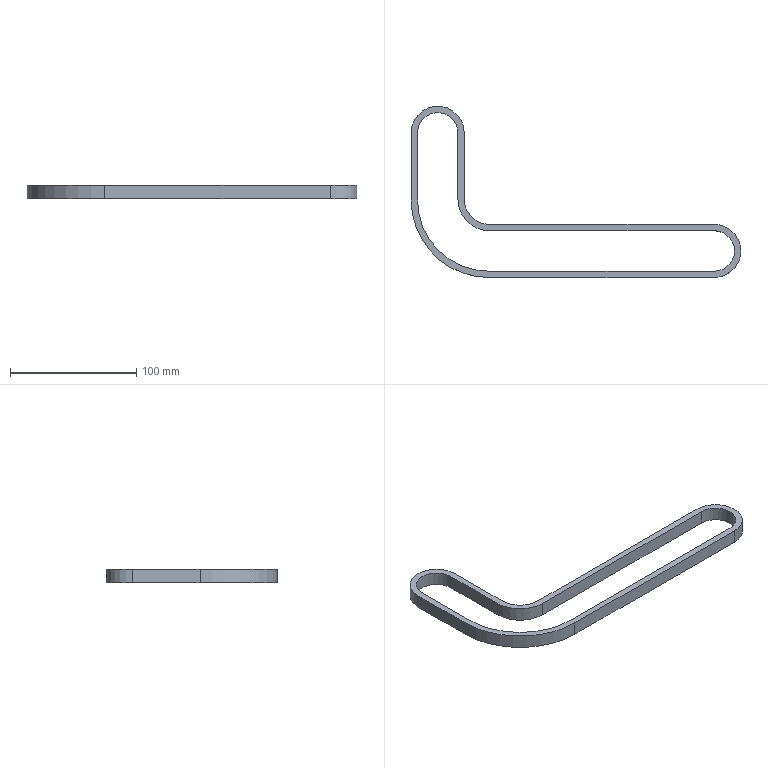Part | SolidWorks | features Extrusion 1 | 1 solid | 20 faces | box 260.844 x 135.477 x 11 mm | volume 38829 mm3 | cylinder 10 | plane 10 | commonest cylinder face diameters 32 x3 42 x3 40 x1 50 x1 112.653 x1 122.653 x1
STEP:
#1=CARTESIAN_POINT('',(195.481,-17.619,-11.));
#2=VERTEX_POINT('',#1);
#3=CARTESIAN_POINT('',(179.481,-1.619,-11.));
#4=VERTEX_POINT('',#3);
#5=CARTESIAN_POINT('',(179.481,-17.619,-11.));
#6=DIRECTION('',(0.,0.,1.));
#7=DIRECTION('',(-1.,0.,0.));
#8=AXIS2_PLACEMENT_3D('',#5,#6,#7);
#9=CIRCLE('',#8,16.);
#10=EDGE_CURVE('',#2,#4,#9,.T.);
#11=ORIENTED_EDGE('',*,*,#10,.F.);
#12=CARTESIAN_POINT('',(195.481,-17.619,0.));
#13=VERTEX_POINT('',#12);
#14=CARTESIAN_POINT('',(195.481,-17.619,-11.));
#15=DIRECTION('',(0.,0.,1.));
#16=VECTOR('',#15,1000.);
#17=LINE('',#14,#16);
#18=EDGE_CURVE('',#2,#13,#17,.T.);
#19=ORIENTED_EDGE('',*,*,#18,.T.);
#20=CARTESIAN_POINT('',(179.481,-1.619,0.));
#21=VERTEX_POINT('',#20);
#22=CARTESIAN_POINT('',(179.481,-17.619,0.));
#23=DIRECTION('',(0.,0.,1.));
#24=DIRECTION('',(-1.,0.,0.));
#25=AXIS2_PLACEMENT_3D('',#22,#23,#24);
#26=CIRCLE('',#25,16.);
#27=EDGE_CURVE('',#13,#21,#26,.T.);
#28=ORIENTED_EDGE('',*,*,#27,.T.);
#29=CARTESIAN_POINT('',(179.481,-1.619,-11.));
#30=DIRECTION('',(0.,0.,1.));
#31=VECTOR('',#30,1000.);
#32=LINE('',#29,#31);
#33=EDGE_CURVE('',#4,#21,#32,.T.);
#34=ORIENTED_EDGE('',*,*,#33,.F.);
#35=EDGE_LOOP('',(#11,#19,#28,#34));
#36=FACE_OUTER_BOUND('',#35,.T.);
#37=CARTESIAN_POINT('',(179.481,-17.619,-11.));
#38=DIRECTION('',(0.,0.,1.));
#39=DIRECTION('',(1.,0.,0.));
#40=AXIS2_PLACEMENT_3D('',#37,#38,#39);
#41=CYLINDRICAL_SURFACE('',#40,16.);
#42=ADVANCED_FACE('',(#36),#41,.F.);
#43=CARTESIAN_POINT('',(179.481,-38.619,-11.));
#44=VERTEX_POINT('',#43);
#45=CARTESIAN_POINT('',(200.481,-17.619,-11.));
#46=VERTEX_POINT('',#45);
#47=CARTESIAN_POINT('',(179.481,-17.619,-11.));
#48=DIRECTION('',(0.,0.,1.));
#49=DIRECTION('',(-1.,0.,0.));
#50=AXIS2_PLACEMENT_3D('',#47,#48,#49);
#51=CIRCLE('',#50,21.);
#52=EDGE_CURVE('',#44,#46,#51,.T.);
#53=ORIENTED_EDGE('',*,*,#52,.T.);
#54=CARTESIAN_POINT('',(200.481,-17.619,0.));
#55=VERTEX_POINT('',#54);
#56=CARTESIAN_POINT('',(200.481,-17.619,-11.));
#57=DIRECTION('',(0.,0.,1.));
#58=VECTOR('',#57,1000.);
#59=LINE('',#56,#58);
#60=EDGE_CURVE('',#46,#55,#59,.T.);
#61=ORIENTED_EDGE('',*,*,#60,.T.);
#62=CARTESIAN_POINT('',(179.481,-38.619,0.));
#63=VERTEX_POINT('',#62);
#64=CARTESIAN_POINT('',(179.481,-17.619,0.));
#65=DIRECTION('',(0.,0.,1.));
#66=DIRECTION('',(-1.,0.,0.));
#67=AXIS2_PLACEMENT_3D('',#64,#65,#66);
#68=CIRCLE('',#67,21.);
#69=EDGE_CURVE('',#63,#55,#68,.T.);
#70=ORIENTED_EDGE('',*,*,#69,.F.);
#71=CARTESIAN_POINT('',(179.481,-38.619,-11.));
#72=DIRECTION('',(0.,0.,1.));
#73=VECTOR('',#72,1000.);
#74=LINE('',#71,#73);
#75=EDGE_CURVE('',#44,#63,#74,.T.);
#76=ORIENTED_EDGE('',*,*,#75,.F.);
#77=EDGE_LOOP('',(#53,#61,#70,#76));
#78=FACE_OUTER_BOUND('',#77,.T.);
#79=CARTESIAN_POINT('',(179.481,-17.619,-11.));
#80=DIRECTION('',(0.,0.,1.));
#81=DIRECTION('',(1.,0.,0.));
#82=AXIS2_PLACEMENT_3D('',#79,#80,#81);
#83=CYLINDRICAL_SURFACE('',#82,21.);
#84=ADVANCED_FACE('',(#78),#83,.T.);
#85=CARTESIAN_POINT('',(1.637,3.381,0.));
#86=VERTEX_POINT('',#85);
#87=CARTESIAN_POINT('',(-18.363,23.381,0.));
#88=VERTEX_POINT('',#87);
#89=CARTESIAN_POINT('',(1.637,23.381,0.));
#90=DIRECTION('',(0.,0.,-1.));
#91=DIRECTION('',(-1.,0.,0.));
#92=AXIS2_PLACEMENT_3D('',#89,#90,#91);
#93=CIRCLE('',#92,20.);
#94=EDGE_CURVE('',#86,#88,#93,.T.);
#95=ORIENTED_EDGE('',*,*,#94,.F.);
#96=CARTESIAN_POINT('',(1.637,3.381,-11.));
#97=VERTEX_POINT('',#96);
#98=CARTESIAN_POINT('',(1.637,3.381,-11.));
#99=DIRECTION('',(0.,0.,1.));
#100=VECTOR('',#99,1000.);
#101=LINE('',#98,#100);
#102=EDGE_CURVE('',#97,#86,#101,.T.);
#103=ORIENTED_EDGE('',*,*,#102,.F.);
#104=CARTESIAN_POINT('',(-18.363,23.381,-11.));
#105=VERTEX_POINT('',#104);
#106=CARTESIAN_POINT('',(1.637,23.381,-11.));
#107=DIRECTION('',(0.,0.,-1.));
#108=DIRECTION('',(-1.,0.,0.));
#109=AXIS2_PLACEMENT_3D('',#106,#107,#108);
#110=CIRCLE('',#109,20.);
#111=EDGE_CURVE('',#97,#105,#110,.T.);
#112=ORIENTED_EDGE('',*,*,#111,.T.);
#113=CARTESIAN_POINT('',(-18.363,23.381,-11.));
#114=DIRECTION('',(0.,0.,1.));
#115=VECTOR('',#114,1000.);
#116=LINE('',#113,#115);
#117=EDGE_CURVE('',#105,#88,#116,.T.);
#118=ORIENTED_EDGE('',*,*,#117,.T.);
#119=EDGE_LOOP('',(#95,#103,#112,#118));
#120=FACE_OUTER_BOUND('',#119,.T.);
#121=CARTESIAN_POINT('',(1.637,23.381,-11.));
#122=DIRECTION('',(0.,0.,1.));
#123=DIRECTION('',(1.,0.,0.));
#124=AXIS2_PLACEMENT_3D('',#121,#122,#123);
#125=CYLINDRICAL_SURFACE('',#124,20.);
#126=ADVANCED_FACE('',(#120),#125,.F.);
#127=CARTESIAN_POINT('',(179.481,3.381,0.));
#128=VERTEX_POINT('',#127);
#129=CARTESIAN_POINT('',(179.481,3.381,0.));
#130=DIRECTION('',(-1.,0.,0.));
#131=VECTOR('',#130,1000.);
#132=LINE('',#129,#131);
#133=EDGE_CURVE('',#128,#86,#132,.T.);
#134=ORIENTED_EDGE('',*,*,#133,.F.);
#135=CARTESIAN_POINT('',(179.481,3.381,-11.));
#136=VERTEX_POINT('',#135);
#137=CARTESIAN_POINT('',(179.481,3.381,-11.));
#138=DIRECTION('',(0.,0.,1.));
#139=VECTOR('',#138,1000.);
#140=LINE('',#137,#139);
#141=EDGE_CURVE('',#136,#128,#140,.T.);
#142=ORIENTED_EDGE('',*,*,#141,.F.);
#143=CARTESIAN_POINT('',(179.481,3.381,-11.));
#144=DIRECTION('',(-1.,0.,0.));
#145=VECTOR('',#144,1000.);
#146=LINE('',#143,#145);
#147=EDGE_CURVE('',#136,#97,#146,.T.);
#148=ORIENTED_EDGE('',*,*,#147,.T.);
#149=ORIENTED_EDGE('',*,*,#102,.T.);
#150=EDGE_LOOP('',(#134,#142,#148,#149));
#151=FACE_OUTER_BOUND('',#150,.T.);
#152=CARTESIAN_POINT('',(179.481,3.381,-11.));
#153=DIRECTION('',(0.,1.,0.));
#154=DIRECTION('',(-1.,0.,0.));
#155=AXIS2_PLACEMENT_3D('',#152,#153,#154);
#156=PLANE('',#155);
#157=ADVANCED_FACE('',(#151),#156,.T.);
#158=ORIENTED_EDGE('',*,*,#60,.F.);
#159=CARTESIAN_POINT('',(179.481,-17.619,-11.));
#160=DIRECTION('',(0.,0.,1.));
#161=DIRECTION('',(-1.,0.,0.));
#162=AXIS2_PLACEMENT_3D('',#159,#160,#161);
#163=CIRCLE('',#162,21.);
#164=EDGE_CURVE('',#46,#136,#163,.T.);
#165=ORIENTED_EDGE('',*,*,#164,.T.);
#166=ORIENTED_EDGE('',*,*,#141,.T.);
#167=CARTESIAN_POINT('',(179.481,-17.619,0.));
#168=DIRECTION('',(0.,0.,1.));
#169=DIRECTION('',(-1.,0.,0.));
#170=AXIS2_PLACEMENT_3D('',#167,#168,#169);
#171=CIRCLE('',#170,21.);
#172=EDGE_CURVE('',#55,#128,#171,.T.);
#173=ORIENTED_EDGE('',*,*,#172,.F.);
#174=EDGE_LOOP('',(#158,#165,#166,#173));
#175=FACE_OUTER_BOUND('',#174,.T.);
#176=CARTESIAN_POINT('',(179.481,-17.619,-11.));
#177=DIRECTION('',(0.,0.,1.));
#178=DIRECTION('',(1.,0.,0.));
#179=AXIS2_PLACEMENT_3D('',#176,#177,#178);
#180=CYLINDRICAL_SURFACE('',#179,21.);
#181=ADVANCED_FACE('',(#175),#180,.T.);
#182=CARTESIAN_POINT('',(0.9629,-38.619,0.));
#183=VERTEX_POINT('',#182);
#184=CARTESIAN_POINT('',(0.9629,-38.619,0.));
#185=DIRECTION('',(1.,0.,0.));
#186=VECTOR('',#185,1000.);
#187=LINE('',#184,#186);
#188=EDGE_CURVE('',#183,#63,#187,.T.);
#189=ORIENTED_EDGE('',*,*,#188,.F.);
#190=CARTESIAN_POINT('',(0.9629,-38.619,-11.));
#191=VERTEX_POINT('',#190);
#192=CARTESIAN_POINT('',(0.9629,-38.619,-11.));
#193=DIRECTION('',(0.,0.,1.));
#194=VECTOR('',#193,1000.);
#195=LINE('',#192,#194);
#196=EDGE_CURVE('',#191,#183,#195,.T.);
#197=ORIENTED_EDGE('',*,*,#196,.F.);
#198=CARTESIAN_POINT('',(0.9629,-38.619,-11.));
#199=DIRECTION('',(1.,0.,0.));
#200=VECTOR('',#199,1000.);
#201=LINE('',#198,#200);
#202=EDGE_CURVE('',#191,#44,#201,.T.);
#203=ORIENTED_EDGE('',*,*,#202,.T.);
#204=ORIENTED_EDGE('',*,*,#75,.T.);
#205=EDGE_LOOP('',(#189,#197,#203,#204));
#206=FACE_OUTER_BOUND('',#205,.T.);
#207=CARTESIAN_POINT('',(0.9629,-38.619,-11.));
#208=DIRECTION('',(0.,-1.,0.));
#209=DIRECTION('',(0.,0.,-1.));
#210=AXIS2_PLACEMENT_3D('',#207,#208,#209);
#211=PLANE('',#210);
#212=ADVANCED_FACE('',(#206),#211,.T.);
#213=CARTESIAN_POINT('',(-60.363,22.707,0.));
#214=VERTEX_POINT('',#213);
#215=CARTESIAN_POINT('',(0.9629,22.707,0.));
#216=DIRECTION('',(0.,0.,1.));
#217=DIRECTION('',(1.,0.,0.));
#218=AXIS2_PLACEMENT_3D('',#215,#216,#217);
#219=CIRCLE('',#218,61.326);
#220=EDGE_CURVE('',#214,#183,#219,.T.);
#221=ORIENTED_EDGE('',*,*,#220,.F.);
#222=CARTESIAN_POINT('',(-60.363,22.707,-11.));
#223=VERTEX_POINT('',#222);
#224=CARTESIAN_POINT('',(-60.363,22.707,-11.));
#225=DIRECTION('',(0.,0.,1.));
#226=VECTOR('',#225,1000.);
#227=LINE('',#224,#226);
#228=EDGE_CURVE('',#223,#214,#227,.T.);
#229=ORIENTED_EDGE('',*,*,#228,.F.);
#230=CARTESIAN_POINT('',(0.9629,22.707,-11.));
#231=DIRECTION('',(0.,0.,1.));
#232=DIRECTION('',(1.,0.,0.));
#233=AXIS2_PLACEMENT_3D('',#230,#231,#232);
#234=CIRCLE('',#233,61.326);
#235=EDGE_CURVE('',#223,#191,#234,.T.);
#236=ORIENTED_EDGE('',*,*,#235,.T.);
#237=ORIENTED_EDGE('',*,*,#196,.T.);
#238=EDGE_LOOP('',(#221,#229,#236,#237));
#239=FACE_OUTER_BOUND('',#238,.T.);
#240=CARTESIAN_POINT('',(0.9629,22.707,-11.));
#241=DIRECTION('',(0.,0.,1.));
#242=DIRECTION('',(1.,0.,0.));
#243=AXIS2_PLACEMENT_3D('',#240,#241,#242);
#244=CYLINDRICAL_SURFACE('',#243,61.326);
#245=ADVANCED_FACE('',(#239),#244,.T.);
#246=CARTESIAN_POINT('',(-60.363,75.858,0.));
#247=VERTEX_POINT('',#246);
#248=CARTESIAN_POINT('',(-60.363,75.858,0.));
#249=DIRECTION('',(0.,-1.,0.));
#250=VECTOR('',#249,1000.);
#251=LINE('',#248,#250);
#252=EDGE_CURVE('',#247,#214,#251,.T.);
#253=ORIENTED_EDGE('',*,*,#252,.F.);
#254=CARTESIAN_POINT('',(-60.363,75.858,-11.));
#255=VERTEX_POINT('',#254);
#256=CARTESIAN_POINT('',(-60.363,75.858,-11.));
#257=DIRECTION('',(0.,0.,1.));
#258=VECTOR('',#257,1000.);
#259=LINE('',#256,#258);
#260=EDGE_CURVE('',#255,#247,#259,.T.);
#261=ORIENTED_EDGE('',*,*,#260,.F.);
#262=CARTESIAN_POINT('',(-60.363,75.858,-11.));
#263=DIRECTION('',(0.,-1.,0.));
#264=VECTOR('',#263,1000.);
#265=LINE('',#262,#264);
#266=EDGE_CURVE('',#255,#223,#265,.T.);
#267=ORIENTED_EDGE('',*,*,#266,.T.);
#268=ORIENTED_EDGE('',*,*,#228,.T.);
#269=EDGE_LOOP('',(#253,#261,#267,#268));
#270=FACE_OUTER_BOUND('',#269,.T.);
#271=CARTESIAN_POINT('',(-60.363,75.858,-11.));
#272=DIRECTION('',(-1.,0.,0.));
#273=DIRECTION('',(0.,-1.,0.));
#274=AXIS2_PLACEMENT_3D('',#271,#272,#273);
#275=PLANE('',#274);
#276=ADVANCED_FACE('',(#270),#275,.T.);
#277=CARTESIAN_POINT('',(-18.363,75.858,0.));
#278=VERTEX_POINT('',#277);
#279=CARTESIAN_POINT('',(-39.363,75.858,0.));
#280=DIRECTION('',(0.,0.,1.));
#281=DIRECTION('',(-1.,0.,0.));
#282=AXIS2_PLACEMENT_3D('',#279,#280,#281);
#283=CIRCLE('',#282,21.);
#284=EDGE_CURVE('',#278,#247,#283,.T.);
#285=ORIENTED_EDGE('',*,*,#284,.F.);
#286=CARTESIAN_POINT('',(-18.363,75.858,-11.));
#287=VERTEX_POINT('',#286);
#288=CARTESIAN_POINT('',(-18.363,75.858,-11.));
#289=DIRECTION('',(0.,0.,1.));
#290=VECTOR('',#289,1000.);
#291=LINE('',#288,#290);
#292=EDGE_CURVE('',#287,#278,#291,.T.);
#293=ORIENTED_EDGE('',*,*,#292,.F.);
#294=CARTESIAN_POINT('',(-39.363,75.858,-11.));
#295=DIRECTION('',(0.,0.,1.));
#296=DIRECTION('',(-1.,0.,0.));
#297=AXIS2_PLACEMENT_3D('',#294,#295,#296);
#298=CIRCLE('',#297,21.);
#299=EDGE_CURVE('',#287,#255,#298,.T.);
#300=ORIENTED_EDGE('',*,*,#299,.T.);
#301=ORIENTED_EDGE('',*,*,#260,.T.);
#302=EDGE_LOOP('',(#285,#293,#300,#301));
#303=FACE_OUTER_BOUND('',#302,.T.);
#304=CARTESIAN_POINT('',(-39.363,75.858,-11.));
#305=DIRECTION('',(0.,0.,1.));
#306=DIRECTION('',(1.,0.,0.));
#307=AXIS2_PLACEMENT_3D('',#304,#305,#306);
#308=CYLINDRICAL_SURFACE('',#307,21.);
#309=ADVANCED_FACE('',(#303),#308,.T.);
#310=CARTESIAN_POINT('',(-18.363,23.381,0.));
#311=DIRECTION('',(0.,1.,0.));
#312=VECTOR('',#311,1000.);
#313=LINE('',#310,#312);
#314=EDGE_CURVE('',#88,#278,#313,.T.);
#315=ORIENTED_EDGE('',*,*,#314,.F.);
#316=ORIENTED_EDGE('',*,*,#117,.F.);
#317=CARTESIAN_POINT('',(-18.363,23.381,-11.));
#318=DIRECTION('',(0.,1.,0.));
#319=VECTOR('',#318,1000.);
#320=LINE('',#317,#319);
#321=EDGE_CURVE('',#105,#287,#320,.T.);
#322=ORIENTED_EDGE('',*,*,#321,.T.);
#323=ORIENTED_EDGE('',*,*,#292,.T.);
#324=EDGE_LOOP('',(#315,#316,#322,#323));
#325=FACE_OUTER_BOUND('',#324,.T.);
#326=CARTESIAN_POINT('',(-18.363,23.381,-11.));
#327=DIRECTION('',(1.,0.,0.));
#328=DIRECTION('',(0.,1.,0.));
#329=AXIS2_PLACEMENT_3D('',#326,#327,#328);
#330=PLANE('',#329);
#331=ADVANCED_FACE('',(#325),#330,.T.);
#332=CARTESIAN_POINT('',(1.637,-1.619,-11.));
#333=VERTEX_POINT('',#332);
#334=CARTESIAN_POINT('',(-23.363,23.381,-11.));
#335=VERTEX_POINT('',#334);
#336=CARTESIAN_POINT('',(1.637,23.381,-11.));
#337=DIRECTION('',(0.,0.,-1.));
#338=DIRECTION('',(-1.,0.,0.));
#339=AXIS2_PLACEMENT_3D('',#336,#337,#338);
#340=CIRCLE('',#339,25.);
#341=EDGE_CURVE('',#333,#335,#340,.T.);
#342=ORIENTED_EDGE('',*,*,#341,.T.);
#343=CARTESIAN_POINT('',(-23.363,75.858,-11.));
#344=VERTEX_POINT('',#343);
#345=CARTESIAN_POINT('',(-23.363,23.381,-11.));
#346=DIRECTION('',(0.,1.,0.));
#347=VECTOR('',#346,1000.);
#348=LINE('',#345,#347);
#349=EDGE_CURVE('',#335,#344,#348,.T.);
#350=ORIENTED_EDGE('',*,*,#349,.T.);
#351=CARTESIAN_POINT('',(-55.363,75.858,-11.));
#352=VERTEX_POINT('',#351);
#353=CARTESIAN_POINT('',(-39.363,75.858,-11.));
#354=DIRECTION('',(0.,0.,1.));
#355=DIRECTION('',(-1.,0.,0.));
#356=AXIS2_PLACEMENT_3D('',#353,#354,#355);
#357=CIRCLE('',#356,16.);
#358=EDGE_CURVE('',#344,#352,#357,.T.);
#359=ORIENTED_EDGE('',*,*,#358,.T.);
#360=CARTESIAN_POINT('',(-55.363,22.707,-11.));
#361=VERTEX_POINT('',#360);
#362=CARTESIAN_POINT('',(-55.363,75.858,-11.));
#363=DIRECTION('',(0.,-1.,0.));
#364=VECTOR('',#363,1000.);
#365=LINE('',#362,#364);
#366=EDGE_CURVE('',#352,#361,#365,.T.);
#367=ORIENTED_EDGE('',*,*,#366,.T.);
#368=CARTESIAN_POINT('',(0.9629,-33.619,-11.));
#369=VERTEX_POINT('',#368);
#370=CARTESIAN_POINT('',(0.9629,22.707,-11.));
#371=DIRECTION('',(0.,0.,1.));
#372=DIRECTION('',(1.,0.,0.));
#373=AXIS2_PLACEMENT_3D('',#370,#371,#372);
#374=CIRCLE('',#373,56.326);
#375=EDGE_CURVE('',#361,#369,#374,.T.);
#376=ORIENTED_EDGE('',*,*,#375,.T.);
#377=CARTESIAN_POINT('',(179.481,-33.619,-11.));
#378=VERTEX_POINT('',#377);
#379=CARTESIAN_POINT('',(0.9629,-33.619,-11.));
#380=DIRECTION('',(1.,0.,0.));
#381=VECTOR('',#380,1000.);
#382=LINE('',#379,#381);
#383=EDGE_CURVE('',#369,#378,#382,.T.);
#384=ORIENTED_EDGE('',*,*,#383,.T.);
#385=CARTESIAN_POINT('',(179.481,-17.619,-11.));
#386=DIRECTION('',(0.,0.,1.));
#387=DIRECTION('',(-1.,0.,0.));
#388=AXIS2_PLACEMENT_3D('',#385,#386,#387);
#389=CIRCLE('',#388,16.);
#390=EDGE_CURVE('',#378,#2,#389,.T.);
#391=ORIENTED_EDGE('',*,*,#390,.T.);
#392=ORIENTED_EDGE('',*,*,#10,.T.);
#393=CARTESIAN_POINT('',(179.481,-1.619,-11.));
#394=DIRECTION('',(-1.,0.,0.));
#395=VECTOR('',#394,1000.);
#396=LINE('',#393,#395);
#397=EDGE_CURVE('',#4,#333,#396,.T.);
#398=ORIENTED_EDGE('',*,*,#397,.T.);
#399=EDGE_LOOP('',(#342,#350,#359,#367,#376,#384,#391,#392,#398));
#400=FACE_BOUND('',#399,.T.);
#401=ORIENTED_EDGE('',*,*,#111,.F.);
#402=ORIENTED_EDGE('',*,*,#147,.F.);
#403=ORIENTED_EDGE('',*,*,#164,.F.);
#404=ORIENTED_EDGE('',*,*,#52,.F.);
#405=ORIENTED_EDGE('',*,*,#202,.F.);
#406=ORIENTED_EDGE('',*,*,#235,.F.);
#407=ORIENTED_EDGE('',*,*,#266,.F.);
#408=ORIENTED_EDGE('',*,*,#299,.F.);
#409=ORIENTED_EDGE('',*,*,#321,.F.);
#410=EDGE_LOOP('',(#401,#402,#403,#404,#405,#406,#407,#408,#409));
#411=FACE_OUTER_BOUND('',#410,.T.);
#412=CARTESIAN_POINT('',(1.637,23.381,-11.));
#413=DIRECTION('',(0.,0.,-1.));
#414=DIRECTION('',(-1.,0.,0.));
#415=AXIS2_PLACEMENT_3D('',#412,#413,#414);
#416=PLANE('',#415);
#417=ADVANCED_FACE('',(#400,#411),#416,.T.);
#418=CARTESIAN_POINT('',(-23.363,23.381,0.));
#419=VERTEX_POINT('',#418);
#420=CARTESIAN_POINT('',(-23.363,75.858,0.));
#421=VERTEX_POINT('',#420);
#422=CARTESIAN_POINT('',(-23.363,23.381,0.));
#423=DIRECTION('',(0.,1.,0.));
#424=VECTOR('',#423,1000.);
#425=LINE('',#422,#424);
#426=EDGE_CURVE('',#419,#421,#425,.T.);
#427=ORIENTED_EDGE('',*,*,#426,.F.);
#428=CARTESIAN_POINT('',(1.637,-1.619,0.));
#429=VERTEX_POINT('',#428);
#430=CARTESIAN_POINT('',(1.637,23.381,0.));
#431=DIRECTION('',(0.,0.,-1.));
#432=DIRECTION('',(-1.,0.,0.));
#433=AXIS2_PLACEMENT_3D('',#430,#431,#432);
#434=CIRCLE('',#433,25.);
#435=EDGE_CURVE('',#429,#419,#434,.T.);
#436=ORIENTED_EDGE('',*,*,#435,.F.);
#437=CARTESIAN_POINT('',(179.481,-1.619,0.));
#438=DIRECTION('',(-1.,0.,0.));
#439=VECTOR('',#438,1000.);
#440=LINE('',#437,#439);
#441=EDGE_CURVE('',#21,#429,#440,.T.);
#442=ORIENTED_EDGE('',*,*,#441,.F.);
#443=ORIENTED_EDGE('',*,*,#27,.F.);
#444=CARTESIAN_POINT('',(179.481,-33.619,0.));
#445=VERTEX_POINT('',#444);
#446=CARTESIAN_POINT('',(179.481,-17.619,0.));
#447=DIRECTION('',(0.,0.,1.));
#448=DIRECTION('',(-1.,0.,0.));
#449=AXIS2_PLACEMENT_3D('',#446,#447,#448);
#450=CIRCLE('',#449,16.);
#451=EDGE_CURVE('',#445,#13,#450,.T.);
#452=ORIENTED_EDGE('',*,*,#451,.F.);
#453=CARTESIAN_POINT('',(0.9629,-33.619,0.));
#454=VERTEX_POINT('',#453);
#455=CARTESIAN_POINT('',(0.9629,-33.619,0.));
#456=DIRECTION('',(1.,0.,0.));
#457=VECTOR('',#456,1000.);
#458=LINE('',#455,#457);
#459=EDGE_CURVE('',#454,#445,#458,.T.);
#460=ORIENTED_EDGE('',*,*,#459,.F.);
#461=CARTESIAN_POINT('',(-55.363,22.707,0.));
#462=VERTEX_POINT('',#461);
#463=CARTESIAN_POINT('',(0.9629,22.707,0.));
#464=DIRECTION('',(0.,0.,1.));
#465=DIRECTION('',(1.,0.,0.));
#466=AXIS2_PLACEMENT_3D('',#463,#464,#465);
#467=CIRCLE('',#466,56.326);
#468=EDGE_CURVE('',#462,#454,#467,.T.);
#469=ORIENTED_EDGE('',*,*,#468,.F.);
#470=CARTESIAN_POINT('',(-55.363,75.858,0.));
#471=VERTEX_POINT('',#470);
#472=CARTESIAN_POINT('',(-55.363,75.858,0.));
#473=DIRECTION('',(0.,-1.,0.));
#474=VECTOR('',#473,1000.);
#475=LINE('',#472,#474);
#476=EDGE_CURVE('',#471,#462,#475,.T.);
#477=ORIENTED_EDGE('',*,*,#476,.F.);
#478=CARTESIAN_POINT('',(-39.363,75.858,0.));
#479=DIRECTION('',(0.,0.,1.));
#480=DIRECTION('',(-1.,0.,0.));
#481=AXIS2_PLACEMENT_3D('',#478,#479,#480);
#482=CIRCLE('',#481,16.);
#483=EDGE_CURVE('',#421,#471,#482,.T.);
#484=ORIENTED_EDGE('',*,*,#483,.F.);
#485=EDGE_LOOP('',(#427,#436,#442,#443,#452,#460,#469,#477,#484));
#486=FACE_BOUND('',#485,.T.);
#487=ORIENTED_EDGE('',*,*,#94,.T.);
#488=ORIENTED_EDGE('',*,*,#314,.T.);
#489=ORIENTED_EDGE('',*,*,#284,.T.);
#490=ORIENTED_EDGE('',*,*,#252,.T.);
#491=ORIENTED_EDGE('',*,*,#220,.T.);
#492=ORIENTED_EDGE('',*,*,#188,.T.);
#493=ORIENTED_EDGE('',*,*,#69,.T.);
#494=ORIENTED_EDGE('',*,*,#172,.T.);
#495=ORIENTED_EDGE('',*,*,#133,.T.);
#496=EDGE_LOOP('',(#487,#488,#489,#490,#491,#492,#493,#494,#495));
#497=FACE_OUTER_BOUND('',#496,.T.);
#498=CARTESIAN_POINT('',(1.637,23.381,0.));
#499=DIRECTION('',(0.,0.,-1.));
#500=DIRECTION('',(-1.,0.,0.));
#501=AXIS2_PLACEMENT_3D('',#498,#499,#500);
#502=PLANE('',#501);
#503=ADVANCED_FACE('',(#486,#497),#502,.F.);
#504=ORIENTED_EDGE('',*,*,#435,.T.);
#505=CARTESIAN_POINT('',(-23.363,23.381,-11.));
#506=DIRECTION('',(0.,0.,1.));
#507=VECTOR('',#506,1000.);
#508=LINE('',#505,#507);
#509=EDGE_CURVE('',#335,#419,#508,.T.);
#510=ORIENTED_EDGE('',*,*,#509,.F.);
#511=ORIENTED_EDGE('',*,*,#341,.F.);
#512=CARTESIAN_POINT('',(1.637,-1.619,-11.));
#513=DIRECTION('',(0.,0.,1.));
#514=VECTOR('',#513,1000.);
#515=LINE('',#512,#514);
#516=EDGE_CURVE('',#333,#429,#515,.T.);
#517=ORIENTED_EDGE('',*,*,#516,.T.);
#518=EDGE_LOOP('',(#504,#510,#511,#517));
#519=FACE_OUTER_BOUND('',#518,.T.);
#520=CARTESIAN_POINT('',(1.637,23.381,-11.));
#521=DIRECTION('',(0.,0.,1.));
#522=DIRECTION('',(1.,0.,0.));
#523=AXIS2_PLACEMENT_3D('',#520,#521,#522);
#524=CYLINDRICAL_SURFACE('',#523,25.);
#525=ADVANCED_FACE('',(#519),#524,.T.);
#526=ORIENTED_EDGE('',*,*,#441,.T.);
#527=ORIENTED_EDGE('',*,*,#516,.F.);
#528=ORIENTED_EDGE('',*,*,#397,.F.);
#529=ORIENTED_EDGE('',*,*,#33,.T.);
#530=EDGE_LOOP('',(#526,#527,#528,#529));
#531=FACE_OUTER_BOUND('',#530,.T.);
#532=CARTESIAN_POINT('',(179.481,-1.619,-11.));
#533=DIRECTION('',(0.,1.,0.));
#534=DIRECTION('',(-1.,0.,0.));
#535=AXIS2_PLACEMENT_3D('',#532,#533,#534);
#536=PLANE('',#535);
#537=ADVANCED_FACE('',(#531),#536,.F.);
#538=ORIENTED_EDGE('',*,*,#18,.F.);
#539=ORIENTED_EDGE('',*,*,#390,.F.);
#540=CARTESIAN_POINT('',(179.481,-33.619,-11.));
#541=DIRECTION('',(0.,0.,1.));
#542=VECTOR('',#541,1000.);
#543=LINE('',#540,#542);
#544=EDGE_CURVE('',#378,#445,#543,.T.);
#545=ORIENTED_EDGE('',*,*,#544,.T.);
#546=ORIENTED_EDGE('',*,*,#451,.T.);
#547=EDGE_LOOP('',(#538,#539,#545,#546));
#548=FACE_OUTER_BOUND('',#547,.T.);
#549=CARTESIAN_POINT('',(179.481,-17.619,-11.));
#550=DIRECTION('',(0.,0.,1.));
#551=DIRECTION('',(1.,0.,0.));
#552=AXIS2_PLACEMENT_3D('',#549,#550,#551);
#553=CYLINDRICAL_SURFACE('',#552,16.);
#554=ADVANCED_FACE('',(#548),#553,.F.);
#555=ORIENTED_EDGE('',*,*,#459,.T.);
#556=ORIENTED_EDGE('',*,*,#544,.F.);
#557=ORIENTED_EDGE('',*,*,#383,.F.);
#558=CARTESIAN_POINT('',(0.9629,-33.619,-11.));
#559=DIRECTION('',(0.,0.,1.));
#560=VECTOR('',#559,1000.);
#561=LINE('',#558,#560);
#562=EDGE_CURVE('',#369,#454,#561,.T.);
#563=ORIENTED_EDGE('',*,*,#562,.T.);
#564=EDGE_LOOP('',(#555,#556,#557,#563));
#565=FACE_OUTER_BOUND('',#564,.T.);
#566=CARTESIAN_POINT('',(0.9629,-33.619,-11.));
#567=DIRECTION('',(0.,-1.,0.));
#568=DIRECTION('',(0.,0.,-1.));
#569=AXIS2_PLACEMENT_3D('',#566,#567,#568);
#570=PLANE('',#569);
#571=ADVANCED_FACE('',(#565),#570,.F.);
#572=ORIENTED_EDGE('',*,*,#468,.T.);
#573=ORIENTED_EDGE('',*,*,#562,.F.);
#574=ORIENTED_EDGE('',*,*,#375,.F.);
#575=CARTESIAN_POINT('',(-55.363,22.707,-11.));
#576=DIRECTION('',(0.,0.,1.));
#577=VECTOR('',#576,1000.);
#578=LINE('',#575,#577);
#579=EDGE_CURVE('',#361,#462,#578,.T.);
#580=ORIENTED_EDGE('',*,*,#579,.T.);
#581=EDGE_LOOP('',(#572,#573,#574,#580));
#582=FACE_OUTER_BOUND('',#581,.T.);
#583=CARTESIAN_POINT('',(0.9629,22.707,-11.));
#584=DIRECTION('',(0.,0.,1.));
#585=DIRECTION('',(1.,0.,0.));
#586=AXIS2_PLACEMENT_3D('',#583,#584,#585);
#587=CYLINDRICAL_SURFACE('',#586,56.326);
#588=ADVANCED_FACE('',(#582),#587,.F.);
#589=ORIENTED_EDGE('',*,*,#476,.T.);
#590=ORIENTED_EDGE('',*,*,#579,.F.);
#591=ORIENTED_EDGE('',*,*,#366,.F.);
#592=CARTESIAN_POINT('',(-55.363,75.858,-11.));
#593=DIRECTION('',(0.,0.,1.));
#594=VECTOR('',#593,1000.);
#595=LINE('',#592,#594);
#596=EDGE_CURVE('',#352,#471,#595,.T.);
#597=ORIENTED_EDGE('',*,*,#596,.T.);
#598=EDGE_LOOP('',(#589,#590,#591,#597));
#599=FACE_OUTER_BOUND('',#598,.T.);
#600=CARTESIAN_POINT('',(-55.363,75.858,-11.));
#601=DIRECTION('',(-1.,0.,0.));
#602=DIRECTION('',(0.,0.,1.));
#603=AXIS2_PLACEMENT_3D('',#600,#601,#602);
#604=PLANE('',#603);
#605=ADVANCED_FACE('',(#599),#604,.F.);
#606=ORIENTED_EDGE('',*,*,#483,.T.);
#607=ORIENTED_EDGE('',*,*,#596,.F.);
#608=ORIENTED_EDGE('',*,*,#358,.F.);
#609=CARTESIAN_POINT('',(-23.363,75.858,-11.));
#610=DIRECTION('',(0.,0.,1.));
#611=VECTOR('',#610,1000.);
#612=LINE('',#609,#611);
#613=EDGE_CURVE('',#344,#421,#612,.T.);
#614=ORIENTED_EDGE('',*,*,#613,.T.);
#615=EDGE_LOOP('',(#606,#607,#608,#614));
#616=FACE_OUTER_BOUND('',#615,.T.);
#617=CARTESIAN_POINT('',(-39.363,75.858,-11.));
#618=DIRECTION('',(0.,0.,1.));
#619=DIRECTION('',(1.,0.,0.));
#620=AXIS2_PLACEMENT_3D('',#617,#618,#619);
#621=CYLINDRICAL_SURFACE('',#620,16.);
#622=ADVANCED_FACE('',(#616),#621,.F.);
#623=ORIENTED_EDGE('',*,*,#426,.T.);
#624=ORIENTED_EDGE('',*,*,#613,.F.);
#625=ORIENTED_EDGE('',*,*,#349,.F.);
#626=ORIENTED_EDGE('',*,*,#509,.T.);
#627=EDGE_LOOP('',(#623,#624,#625,#626));
#628=FACE_OUTER_BOUND('',#627,.T.);
#629=CARTESIAN_POINT('',(-23.363,23.381,-11.));
#630=DIRECTION('',(1.,0.,0.));
#631=DIRECTION('',(0.,1.,0.));
#632=AXIS2_PLACEMENT_3D('',#629,#630,#631);
#633=PLANE('',#632);
#634=ADVANCED_FACE('',(#628),#633,.F.);
#635=CLOSED_SHELL('',(#42,#84,#126,#157,#181,#212,#245,#276,#309,#331,#417,#503,#525,#537,#554,#571,#588,#605,#622,#634));
#636=MANIFOLD_SOLID_BREP('',#635);
#637=CARTESIAN_POINT('',(0.,0.,0.));
#638=DIRECTION('',(0.,0.,1.));
#639=DIRECTION('',(1.,0.,0.));
#640=AXIS2_PLACEMENT_3D('',#637,#638,#639);
#641=(LENGTH_UNIT()NAMED_UNIT(*)SI_UNIT(.MILLI.,.METRE.));
#642=UNCERTAINTY_MEASURE_WITH_UNIT(LENGTH_MEASURE(0.00001),#641,'','');
#643=(NAMED_UNIT(*)PLANE_ANGLE_UNIT()SI_UNIT($,.RADIAN.));
#644=(NAMED_UNIT(*)SI_UNIT($,.STERADIAN.)SOLID_ANGLE_UNIT());
#645=(GEOMETRIC_REPRESENTATION_CONTEXT(3)GLOBAL_UNCERTAINTY_ASSIGNED_CONTEXT((#642))GLOBAL_UNIT_ASSIGNED_CONTEXT((#641,#643,#644))REPRESENTATION_CONTEXT('',''));
#646=ADVANCED_BREP_SHAPE_REPRESENTATION('',(#636,#640),#645);